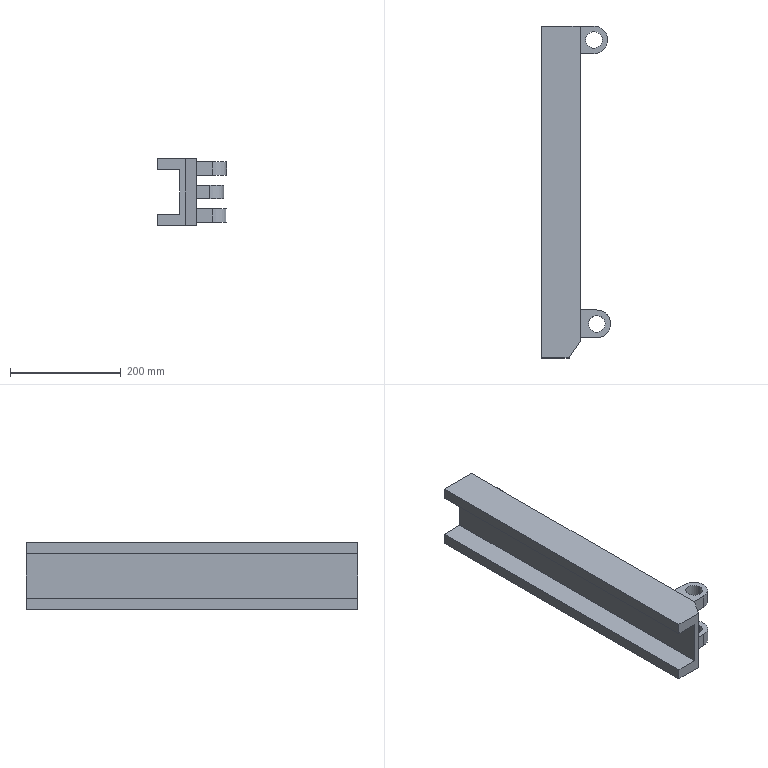Part | SolidWorks | features ICE 4, MirrorPattern 2, Extrusion 1 | 1 solid | 33 faces | box 125 x 600 x 120 mm | volume 3208933 mm3 | plane 22 | cylinder 11 | commonest cylinder face diameters 30 x6 50 x5
STEP:
#1=CARTESIAN_POINT('',(60.,575.,-12.));
#2=VERTEX_POINT('',#1);
#3=CARTESIAN_POINT('',(90.,575.,-12.));
#4=VERTEX_POINT('',#3);
#5=CARTESIAN_POINT('',(75.,575.,-12.));
#6=DIRECTION('',(0.,0.,1.));
#7=DIRECTION('',(1.,0.,0.));
#8=AXIS2_PLACEMENT_3D('',#5,#6,#7);
#9=CIRCLE('',#8,15.);
#10=EDGE_CURVE('',#2,#4,#9,.T.);
#11=ORIENTED_EDGE('',*,*,#10,.F.);
#12=CARTESIAN_POINT('',(60.,575.,12.));
#13=VERTEX_POINT('',#12);
#14=CARTESIAN_POINT('',(60.,575.,-12.));
#15=DIRECTION('',(0.,0.,1.));
#16=VECTOR('',#15,1000.);
#17=LINE('',#14,#16);
#18=EDGE_CURVE('',#2,#13,#17,.T.);
#19=ORIENTED_EDGE('',*,*,#18,.T.);
#20=CARTESIAN_POINT('',(90.,575.,12.));
#21=VERTEX_POINT('',#20);
#22=CARTESIAN_POINT('',(75.,575.,12.));
#23=DIRECTION('',(0.,0.,1.));
#24=DIRECTION('',(1.,0.,0.));
#25=AXIS2_PLACEMENT_3D('',#22,#23,#24);
#26=CIRCLE('',#25,15.);
#27=EDGE_CURVE('',#13,#21,#26,.T.);
#28=ORIENTED_EDGE('',*,*,#27,.T.);
#29=CARTESIAN_POINT('',(90.,575.,-12.));
#30=DIRECTION('',(0.,0.,1.));
#31=VECTOR('',#30,1000.);
#32=LINE('',#29,#31);
#33=EDGE_CURVE('',#4,#21,#32,.T.);
#34=ORIENTED_EDGE('',*,*,#33,.F.);
#35=EDGE_LOOP('',(#11,#19,#28,#34));
#36=FACE_OUTER_BOUND('',#35,.T.);
#37=CARTESIAN_POINT('',(75.,575.,-12.));
#38=DIRECTION('',(0.,0.,1.));
#39=DIRECTION('',(1.,0.,0.));
#40=AXIS2_PLACEMENT_3D('',#37,#38,#39);
#41=CYLINDRICAL_SURFACE('',#40,15.);
#42=ADVANCED_FACE('',(#36),#41,.F.);
#43=CARTESIAN_POINT('',(75.,550.,-12.));
#44=VERTEX_POINT('',#43);
#45=CARTESIAN_POINT('',(100.,575.,-12.));
#46=VERTEX_POINT('',#45);
#47=CARTESIAN_POINT('',(75.,575.,-12.));
#48=DIRECTION('',(0.,0.,1.));
#49=DIRECTION('',(1.,0.,0.));
#50=AXIS2_PLACEMENT_3D('',#47,#48,#49);
#51=CIRCLE('',#50,25.);
#52=EDGE_CURVE('',#44,#46,#51,.T.);
#53=ORIENTED_EDGE('',*,*,#52,.T.);
#54=CARTESIAN_POINT('',(100.,575.,12.));
#55=VERTEX_POINT('',#54);
#56=CARTESIAN_POINT('',(100.,575.,-12.));
#57=DIRECTION('',(0.,0.,1.));
#58=VECTOR('',#57,1000.);
#59=LINE('',#56,#58);
#60=EDGE_CURVE('',#46,#55,#59,.T.);
#61=ORIENTED_EDGE('',*,*,#60,.T.);
#62=CARTESIAN_POINT('',(75.,550.,12.));
#63=VERTEX_POINT('',#62);
#64=CARTESIAN_POINT('',(75.,575.,12.));
#65=DIRECTION('',(0.,0.,1.));
#66=DIRECTION('',(1.,0.,0.));
#67=AXIS2_PLACEMENT_3D('',#64,#65,#66);
#68=CIRCLE('',#67,25.);
#69=EDGE_CURVE('',#63,#55,#68,.T.);
#70=ORIENTED_EDGE('',*,*,#69,.F.);
#71=CARTESIAN_POINT('',(75.,550.,-12.));
#72=DIRECTION('',(0.,0.,1.));
#73=VECTOR('',#72,1000.);
#74=LINE('',#71,#73);
#75=EDGE_CURVE('',#44,#63,#74,.T.);
#76=ORIENTED_EDGE('',*,*,#75,.F.);
#77=EDGE_LOOP('',(#53,#61,#70,#76));
#78=FACE_OUTER_BOUND('',#77,.T.);
#79=CARTESIAN_POINT('',(75.,575.,-12.));
#80=DIRECTION('',(0.,0.,1.));
#81=DIRECTION('',(1.,0.,0.));
#82=AXIS2_PLACEMENT_3D('',#79,#80,#81);
#83=CYLINDRICAL_SURFACE('',#82,25.);
#84=ADVANCED_FACE('',(#78),#83,.T.);
#85=CARTESIAN_POINT('',(95.,61.654,-30.));
#86=VERTEX_POINT('',#85);
#87=CARTESIAN_POINT('',(65.,61.654,-30.));
#88=VERTEX_POINT('',#87);
#89=CARTESIAN_POINT('',(80.,61.654,-30.));
#90=DIRECTION('',(0.,0.,-1.));
#91=DIRECTION('',(-1.,0.,0.));
#92=AXIS2_PLACEMENT_3D('',#89,#90,#91);
#93=CIRCLE('',#92,15.);
#94=EDGE_CURVE('',#86,#88,#93,.T.);
#95=ORIENTED_EDGE('',*,*,#94,.F.);
#96=CARTESIAN_POINT('',(95.,61.654,-55.));
#97=VERTEX_POINT('',#96);
#98=CARTESIAN_POINT('',(95.,61.654,-30.));
#99=DIRECTION('',(0.,0.,-1.));
#100=VECTOR('',#99,1000.);
#101=LINE('',#98,#100);
#102=EDGE_CURVE('',#86,#97,#101,.T.);
#103=ORIENTED_EDGE('',*,*,#102,.T.);
#104=CARTESIAN_POINT('',(65.,61.654,-55.));
#105=VERTEX_POINT('',#104);
#106=CARTESIAN_POINT('',(80.,61.654,-55.));
#107=DIRECTION('',(0.,0.,1.));
#108=DIRECTION('',(-1.,0.,0.));
#109=AXIS2_PLACEMENT_3D('',#106,#107,#108);
#110=CIRCLE('',#109,15.);
#111=EDGE_CURVE('',#105,#97,#110,.T.);
#112=ORIENTED_EDGE('',*,*,#111,.F.);
#113=CARTESIAN_POINT('',(65.,61.654,-30.));
#114=DIRECTION('',(0.,0.,-1.));
#115=VECTOR('',#114,1000.);
#116=LINE('',#113,#115);
#117=EDGE_CURVE('',#88,#105,#116,.T.);
#118=ORIENTED_EDGE('',*,*,#117,.F.);
#119=EDGE_LOOP('',(#95,#103,#112,#118));
#120=FACE_OUTER_BOUND('',#119,.T.);
#121=CARTESIAN_POINT('',(80.,61.654,-30.));
#122=DIRECTION('',(0.,0.,-1.));
#123=DIRECTION('',(-1.,0.,0.));
#124=AXIS2_PLACEMENT_3D('',#121,#122,#123);
#125=CYLINDRICAL_SURFACE('',#124,15.);
#126=ADVANCED_FACE('',(#120),#125,.F.);
#127=CARTESIAN_POINT('',(95.,61.654,30.));
#128=VERTEX_POINT('',#127);
#129=CARTESIAN_POINT('',(65.,61.654,30.));
#130=VERTEX_POINT('',#129);
#131=CARTESIAN_POINT('',(80.,61.654,30.));
#132=DIRECTION('',(0.,0.,-1.));
#133=DIRECTION('',(-1.,0.,0.));
#134=AXIS2_PLACEMENT_3D('',#131,#132,#133);
#135=CIRCLE('',#134,15.);
#136=EDGE_CURVE('',#128,#130,#135,.T.);
#137=ORIENTED_EDGE('',*,*,#136,.T.);
#138=CARTESIAN_POINT('',(65.,61.654,55.));
#139=VERTEX_POINT('',#138);
#140=CARTESIAN_POINT('',(65.,61.654,30.));
#141=DIRECTION('',(0.,0.,1.));
#142=VECTOR('',#141,1000.);
#143=LINE('',#140,#142);
#144=EDGE_CURVE('',#130,#139,#143,.T.);
#145=ORIENTED_EDGE('',*,*,#144,.T.);
#146=CARTESIAN_POINT('',(95.,61.654,55.));
#147=VERTEX_POINT('',#146);
#148=CARTESIAN_POINT('',(80.,61.654,55.));
#149=DIRECTION('',(0.,0.,1.));
#150=DIRECTION('',(1.,0.,0.));
#151=AXIS2_PLACEMENT_3D('',#148,#149,#150);
#152=CIRCLE('',#151,15.);
#153=EDGE_CURVE('',#139,#147,#152,.T.);
#154=ORIENTED_EDGE('',*,*,#153,.T.);
#155=CARTESIAN_POINT('',(95.,61.654,30.));
#156=DIRECTION('',(0.,0.,1.));
#157=VECTOR('',#156,1000.);
#158=LINE('',#155,#157);
#159=EDGE_CURVE('',#128,#147,#158,.T.);
#160=ORIENTED_EDGE('',*,*,#159,.F.);
#161=EDGE_LOOP('',(#137,#145,#154,#160));
#162=FACE_OUTER_BOUND('',#161,.T.);
#163=CARTESIAN_POINT('',(80.,61.654,30.));
#164=DIRECTION('',(0.,0.,1.));
#165=DIRECTION('',(1.,0.,0.));
#166=AXIS2_PLACEMENT_3D('',#163,#164,#165);
#167=CYLINDRICAL_SURFACE('',#166,15.);
#168=ADVANCED_FACE('',(#162),#167,.F.);
#169=CARTESIAN_POINT('',(105.,61.654,30.));
#170=VERTEX_POINT('',#169);
#171=CARTESIAN_POINT('',(80.,36.654,30.));
#172=VERTEX_POINT('',#171);
#173=CARTESIAN_POINT('',(80.,61.654,30.));
#174=DIRECTION('',(0.,0.,-1.));
#175=DIRECTION('',(-1.,0.,0.));
#176=AXIS2_PLACEMENT_3D('',#173,#174,#175);
#177=CIRCLE('',#176,25.);
#178=EDGE_CURVE('',#170,#172,#177,.T.);
#179=ORIENTED_EDGE('',*,*,#178,.F.);
#180=CARTESIAN_POINT('',(105.,61.654,55.));
#181=VERTEX_POINT('',#180);
#182=CARTESIAN_POINT('',(105.,61.654,30.));
#183=DIRECTION('',(0.,0.,1.));
#184=VECTOR('',#183,1000.);
#185=LINE('',#182,#184);
#186=EDGE_CURVE('',#170,#181,#185,.T.);
#187=ORIENTED_EDGE('',*,*,#186,.T.);
#188=CARTESIAN_POINT('',(80.,36.654,55.));
#189=VERTEX_POINT('',#188);
#190=CARTESIAN_POINT('',(80.,61.654,55.));
#191=DIRECTION('',(0.,0.,1.));
#192=DIRECTION('',(1.,0.,0.));
#193=AXIS2_PLACEMENT_3D('',#190,#191,#192);
#194=CIRCLE('',#193,25.);
#195=EDGE_CURVE('',#189,#181,#194,.T.);
#196=ORIENTED_EDGE('',*,*,#195,.F.);
#197=CARTESIAN_POINT('',(80.,36.654,30.));
#198=DIRECTION('',(0.,0.,1.));
#199=VECTOR('',#198,1000.);
#200=LINE('',#197,#199);
#201=EDGE_CURVE('',#172,#189,#200,.T.);
#202=ORIENTED_EDGE('',*,*,#201,.F.);
#203=EDGE_LOOP('',(#179,#187,#196,#202));
#204=FACE_OUTER_BOUND('',#203,.T.);
#205=CARTESIAN_POINT('',(80.,61.654,30.));
#206=DIRECTION('',(0.,0.,1.));
#207=DIRECTION('',(1.,0.,0.));
#208=AXIS2_PLACEMENT_3D('',#205,#206,#207);
#209=CYLINDRICAL_SURFACE('',#208,25.);
#210=ADVANCED_FACE('',(#204),#209,.T.);
#211=CARTESIAN_POINT('',(-20.,0.,60.));
#212=VERTEX_POINT('',#211);
#213=CARTESIAN_POINT('',(30.,0.,60.));
#214=VERTEX_POINT('',#213);
#215=CARTESIAN_POINT('',(-20.,0.,60.));
#216=DIRECTION('',(1.,0.,0.));
#217=VECTOR('',#216,1000.);
#218=LINE('',#215,#217);
#219=EDGE_CURVE('',#212,#214,#218,.T.);
#220=ORIENTED_EDGE('',*,*,#219,.T.);
#221=CARTESIAN_POINT('',(50.,30.341,60.));
#222=VERTEX_POINT('',#221);
#223=CARTESIAN_POINT('',(50.,30.341,60.));
#224=DIRECTION('',(0.5504,0.8349,0.));
#225=VECTOR('',#224,1000.);
#226=LINE('',#223,#225);
#227=EDGE_CURVE('',#214,#222,#226,.T.);
#228=ORIENTED_EDGE('',*,*,#227,.T.);
#229=CARTESIAN_POINT('',(50.,600.,60.));
#230=VERTEX_POINT('',#229);
#231=CARTESIAN_POINT('',(50.,600.,60.));
#232=DIRECTION('',(0.,-1.,0.));
#233=VECTOR('',#232,1000.);
#234=LINE('',#231,#233);
#235=EDGE_CURVE('',#230,#222,#234,.T.);
#236=ORIENTED_EDGE('',*,*,#235,.F.);
#237=CARTESIAN_POINT('',(-20.,600.,60.));
#238=VERTEX_POINT('',#237);
#239=CARTESIAN_POINT('',(-20.,600.,60.));
#240=DIRECTION('',(1.,0.,0.));
#241=VECTOR('',#240,1000.);
#242=LINE('',#239,#241);
#243=EDGE_CURVE('',#238,#230,#242,.T.);
#244=ORIENTED_EDGE('',*,*,#243,.F.);
#245=CARTESIAN_POINT('',(-20.,600.,60.));
#246=DIRECTION('',(0.,-1.,0.));
#247=VECTOR('',#246,1000.);
#248=LINE('',#245,#247);
#249=EDGE_CURVE('',#238,#212,#248,.T.);
#250=ORIENTED_EDGE('',*,*,#249,.T.);
#251=EDGE_LOOP('',(#220,#228,#236,#244,#250));
#252=FACE_OUTER_BOUND('',#251,.T.);
#253=CARTESIAN_POINT('',(-20.,600.,60.));
#254=DIRECTION('',(0.,0.,-1.));
#255=DIRECTION('',(-1.,0.,0.));
#256=AXIS2_PLACEMENT_3D('',#253,#254,#255);
#257=PLANE('',#256);
#258=ADVANCED_FACE('',(#252),#257,.F.);
#259=CARTESIAN_POINT('',(50.,36.654,55.));
#260=VERTEX_POINT('',#259);
#261=CARTESIAN_POINT('',(50.,36.654,55.));
#262=DIRECTION('',(-1.,0.,0.));
#263=VECTOR('',#262,1000.);
#264=LINE('',#261,#263);
#265=EDGE_CURVE('',#189,#260,#264,.T.);
#266=ORIENTED_EDGE('',*,*,#265,.T.);
#267=CARTESIAN_POINT('',(50.,36.654,30.));
#268=VERTEX_POINT('',#267);
#269=CARTESIAN_POINT('',(50.,36.654,-60.));
#270=DIRECTION('',(0.,0.,-1.));
#271=VECTOR('',#270,1000.);
#272=LINE('',#269,#271);
#273=EDGE_CURVE('',#260,#268,#272,.T.);
#274=ORIENTED_EDGE('',*,*,#273,.T.);
#275=CARTESIAN_POINT('',(34.984,36.654,30.));
#276=DIRECTION('',(-1.,0.,0.));
#277=VECTOR('',#276,1000.);
#278=LINE('',#275,#277);
#279=EDGE_CURVE('',#172,#268,#278,.T.);
#280=ORIENTED_EDGE('',*,*,#279,.F.);
#281=ORIENTED_EDGE('',*,*,#201,.T.);
#282=EDGE_LOOP('',(#266,#274,#280,#281));
#283=FACE_OUTER_BOUND('',#282,.T.);
#284=CARTESIAN_POINT('',(34.984,36.654,30.));
#285=DIRECTION('',(0.,1.,0.));
#286=DIRECTION('',(0.,0.,1.));
#287=AXIS2_PLACEMENT_3D('',#284,#285,#286);
#288=PLANE('',#287);
#289=ADVANCED_FACE('',(#283),#288,.F.);
#290=CARTESIAN_POINT('',(80.,86.654,55.));
#291=VERTEX_POINT('',#290);
#292=CARTESIAN_POINT('',(50.,86.654,55.));
#293=VERTEX_POINT('',#292);
#294=CARTESIAN_POINT('',(34.984,86.654,55.));
#295=DIRECTION('',(-1.,0.,0.));
#296=VECTOR('',#295,1000.);
#297=LINE('',#294,#296);
#298=EDGE_CURVE('',#291,#293,#297,.T.);
#299=ORIENTED_EDGE('',*,*,#298,.F.);
#300=CARTESIAN_POINT('',(80.,86.654,30.));
#301=VERTEX_POINT('',#300);
#302=CARTESIAN_POINT('',(80.,86.654,30.));
#303=DIRECTION('',(0.,0.,1.));
#304=VECTOR('',#303,1000.);
#305=LINE('',#302,#304);
#306=EDGE_CURVE('',#301,#291,#305,.T.);
#307=ORIENTED_EDGE('',*,*,#306,.F.);
#308=CARTESIAN_POINT('',(50.,86.654,30.));
#309=VERTEX_POINT('',#308);
#310=CARTESIAN_POINT('',(34.984,86.654,30.));
#311=DIRECTION('',(1.,0.,0.));
#312=VECTOR('',#311,1000.);
#313=LINE('',#310,#312);
#314=EDGE_CURVE('',#309,#301,#313,.T.);
#315=ORIENTED_EDGE('',*,*,#314,.F.);
#316=CARTESIAN_POINT('',(50.,86.654,-60.));
#317=DIRECTION('',(0.,0.,1.));
#318=VECTOR('',#317,1000.);
#319=LINE('',#316,#318);
#320=EDGE_CURVE('',#309,#293,#319,.T.);
#321=ORIENTED_EDGE('',*,*,#320,.T.);
#322=EDGE_LOOP('',(#299,#307,#315,#321));
#323=FACE_OUTER_BOUND('',#322,.T.);
#324=CARTESIAN_POINT('',(34.984,86.654,30.));
#325=DIRECTION('',(0.,-1.,0.));
#326=DIRECTION('',(0.,0.,-1.));
#327=AXIS2_PLACEMENT_3D('',#324,#325,#326);
#328=PLANE('',#327);
#329=ADVANCED_FACE('',(#323),#328,.F.);
#330=ORIENTED_EDGE('',*,*,#186,.F.);
#331=CARTESIAN_POINT('',(80.,61.654,30.));
#332=DIRECTION('',(0.,0.,-1.));
#333=DIRECTION('',(-1.,0.,0.));
#334=AXIS2_PLACEMENT_3D('',#331,#332,#333);
#335=CIRCLE('',#334,25.);
#336=EDGE_CURVE('',#301,#170,#335,.T.);
#337=ORIENTED_EDGE('',*,*,#336,.F.);
#338=ORIENTED_EDGE('',*,*,#306,.T.);
#339=CARTESIAN_POINT('',(80.,61.654,55.));
#340=DIRECTION('',(0.,0.,1.));
#341=DIRECTION('',(1.,0.,0.));
#342=AXIS2_PLACEMENT_3D('',#339,#340,#341);
#343=CIRCLE('',#342,25.);
#344=EDGE_CURVE('',#181,#291,#343,.T.);
#345=ORIENTED_EDGE('',*,*,#344,.F.);
#346=EDGE_LOOP('',(#330,#337,#338,#345));
#347=FACE_OUTER_BOUND('',#346,.T.);
#348=CARTESIAN_POINT('',(80.,61.654,30.));
#349=DIRECTION('',(0.,0.,1.));
#350=DIRECTION('',(1.,0.,0.));
#351=AXIS2_PLACEMENT_3D('',#348,#349,#350);
#352=CYLINDRICAL_SURFACE('',#351,25.);
#353=ADVANCED_FACE('',(#347),#352,.T.);
#354=ORIENTED_EDGE('',*,*,#144,.F.);
#355=CARTESIAN_POINT('',(80.,61.654,30.));
#356=DIRECTION('',(0.,0.,-1.));
#357=DIRECTION('',(-1.,0.,0.));
#358=AXIS2_PLACEMENT_3D('',#355,#356,#357);
#359=CIRCLE('',#358,15.);
#360=EDGE_CURVE('',#130,#128,#359,.T.);
#361=ORIENTED_EDGE('',*,*,#360,.T.);
#362=ORIENTED_EDGE('',*,*,#159,.T.);
#363=CARTESIAN_POINT('',(80.,61.654,55.));
#364=DIRECTION('',(0.,0.,1.));
#365=DIRECTION('',(1.,0.,0.));
#366=AXIS2_PLACEMENT_3D('',#363,#364,#365);
#367=CIRCLE('',#366,15.);
#368=EDGE_CURVE('',#147,#139,#367,.T.);
#369=ORIENTED_EDGE('',*,*,#368,.T.);
#370=EDGE_LOOP('',(#354,#361,#362,#369));
#371=FACE_OUTER_BOUND('',#370,.T.);
#372=CARTESIAN_POINT('',(80.,61.654,30.));
#373=DIRECTION('',(0.,0.,1.));
#374=DIRECTION('',(1.,0.,0.));
#375=AXIS2_PLACEMENT_3D('',#372,#373,#374);
#376=CYLINDRICAL_SURFACE('',#375,15.);
#377=ADVANCED_FACE('',(#371),#376,.F.);
#378=CARTESIAN_POINT('',(80.,86.654,-30.));
#379=VERTEX_POINT('',#378);
#380=CARTESIAN_POINT('',(80.,86.654,-55.));
#381=VERTEX_POINT('',#380);
#382=CARTESIAN_POINT('',(80.,86.654,-30.));
#383=DIRECTION('',(0.,0.,-1.));
#384=VECTOR('',#383,1000.);
#385=LINE('',#382,#384);
#386=EDGE_CURVE('',#379,#381,#385,.T.);
#387=ORIENTED_EDGE('',*,*,#386,.T.);
#388=CARTESIAN_POINT('',(50.,86.654,-55.));
#389=VERTEX_POINT('',#388);
#390=CARTESIAN_POINT('',(34.984,86.654,-55.));
#391=DIRECTION('',(-1.,0.,0.));
#392=VECTOR('',#391,1000.);
#393=LINE('',#390,#392);
#394=EDGE_CURVE('',#381,#389,#393,.T.);
#395=ORIENTED_EDGE('',*,*,#394,.T.);
#396=CARTESIAN_POINT('',(50.,86.654,-30.));
#397=VERTEX_POINT('',#396);
#398=CARTESIAN_POINT('',(50.,86.654,-60.));
#399=DIRECTION('',(0.,0.,-1.));
#400=VECTOR('',#399,1000.);
#401=LINE('',#398,#400);
#402=EDGE_CURVE('',#397,#389,#401,.T.);
#403=ORIENTED_EDGE('',*,*,#402,.F.);
#404=CARTESIAN_POINT('',(34.984,86.654,-30.));
#405=DIRECTION('',(1.,0.,0.));
#406=VECTOR('',#405,1000.);
#407=LINE('',#404,#406);
#408=EDGE_CURVE('',#397,#379,#407,.T.);
#409=ORIENTED_EDGE('',*,*,#408,.T.);
#410=EDGE_LOOP('',(#387,#395,#403,#409));
#411=FACE_OUTER_BOUND('',#410,.T.);
#412=CARTESIAN_POINT('',(34.984,86.654,-30.));
#413=DIRECTION('',(0.,1.,0.));
#414=DIRECTION('',(0.,0.,1.));
#415=AXIS2_PLACEMENT_3D('',#412,#413,#414);
#416=PLANE('',#415);
#417=ADVANCED_FACE('',(#411),#416,.T.);
#418=CARTESIAN_POINT('',(50.,36.654,-55.));
#419=VERTEX_POINT('',#418);
#420=CARTESIAN_POINT('',(50.,36.654,-30.));
#421=VERTEX_POINT('',#420);
#422=CARTESIAN_POINT('',(50.,36.654,-60.));
#423=DIRECTION('',(0.,0.,1.));
#424=VECTOR('',#423,1000.);
#425=LINE('',#422,#424);
#426=EDGE_CURVE('',#419,#421,#425,.T.);
#427=ORIENTED_EDGE('',*,*,#426,.F.);
#428=CARTESIAN_POINT('',(80.,36.654,-55.));
#429=VERTEX_POINT('',#428);
#430=CARTESIAN_POINT('',(50.,36.654,-55.));
#431=DIRECTION('',(-1.,0.,0.));
#432=VECTOR('',#431,1000.);
#433=LINE('',#430,#432);
#434=EDGE_CURVE('',#429,#419,#433,.T.);
#435=ORIENTED_EDGE('',*,*,#434,.F.);
#436=CARTESIAN_POINT('',(80.,36.654,-30.));
#437=VERTEX_POINT('',#436);
#438=CARTESIAN_POINT('',(80.,36.654,-30.));
#439=DIRECTION('',(0.,0.,-1.));
#440=VECTOR('',#439,1000.);
#441=LINE('',#438,#440);
#442=EDGE_CURVE('',#437,#429,#441,.T.);
#443=ORIENTED_EDGE('',*,*,#442,.F.);
#444=CARTESIAN_POINT('',(34.984,36.654,-30.));
#445=DIRECTION('',(-1.,0.,0.));
#446=VECTOR('',#445,1000.);
#447=LINE('',#444,#446);
#448=EDGE_CURVE('',#437,#421,#447,.T.);
#449=ORIENTED_EDGE('',*,*,#448,.T.);
#450=EDGE_LOOP('',(#427,#435,#443,#449));
#451=FACE_OUTER_BOUND('',#450,.T.);
#452=CARTESIAN_POINT('',(34.984,36.654,-30.));
#453=DIRECTION('',(0.,-1.,0.));
#454=DIRECTION('',(0.,0.,-1.));
#455=AXIS2_PLACEMENT_3D('',#452,#453,#454);
#456=PLANE('',#455);
#457=ADVANCED_FACE('',(#451),#456,.T.);
#458=ORIENTED_EDGE('',*,*,#442,.T.);
#459=CARTESIAN_POINT('',(80.,61.654,-55.));
#460=DIRECTION('',(0.,0.,1.));
#461=DIRECTION('',(-1.,0.,0.));
#462=AXIS2_PLACEMENT_3D('',#459,#460,#461);
#463=CIRCLE('',#462,25.);
#464=EDGE_CURVE('',#429,#381,#463,.T.);
#465=ORIENTED_EDGE('',*,*,#464,.T.);
#466=ORIENTED_EDGE('',*,*,#386,.F.);
#467=CARTESIAN_POINT('',(80.,61.654,-30.));
#468=DIRECTION('',(0.,0.,-1.));
#469=DIRECTION('',(-1.,0.,0.));
#470=AXIS2_PLACEMENT_3D('',#467,#468,#469);
#471=CIRCLE('',#470,25.);
#472=EDGE_CURVE('',#379,#437,#471,.T.);
#473=ORIENTED_EDGE('',*,*,#472,.T.);
#474=EDGE_LOOP('',(#458,#465,#466,#473));
#475=FACE_OUTER_BOUND('',#474,.T.);
#476=CARTESIAN_POINT('',(80.,61.654,-30.));
#477=DIRECTION('',(0.,0.,-1.));
#478=DIRECTION('',(-1.,0.,0.));
#479=AXIS2_PLACEMENT_3D('',#476,#477,#478);
#480=CYLINDRICAL_SURFACE('',#479,25.);
#481=ADVANCED_FACE('',(#475),#480,.T.);
#482=ORIENTED_EDGE('',*,*,#102,.F.);
#483=CARTESIAN_POINT('',(80.,61.654,-30.));
#484=DIRECTION('',(0.,0.,-1.));
#485=DIRECTION('',(-1.,0.,0.));
#486=AXIS2_PLACEMENT_3D('',#483,#484,#485);
#487=CIRCLE('',#486,15.);
#488=EDGE_CURVE('',#88,#86,#487,.T.);
#489=ORIENTED_EDGE('',*,*,#488,.F.);
#490=ORIENTED_EDGE('',*,*,#117,.T.);
#491=CARTESIAN_POINT('',(80.,61.654,-55.));
#492=DIRECTION('',(0.,0.,1.));
#493=DIRECTION('',(-1.,0.,0.));
#494=AXIS2_PLACEMENT_3D('',#491,#492,#493);
#495=CIRCLE('',#494,15.);
#496=EDGE_CURVE('',#97,#105,#495,.T.);
#497=ORIENTED_EDGE('',*,*,#496,.F.);
#498=EDGE_LOOP('',(#482,#489,#490,#497));
#499=FACE_OUTER_BOUND('',#498,.T.);
#500=CARTESIAN_POINT('',(80.,61.654,-30.));
#501=DIRECTION('',(0.,0.,-1.));
#502=DIRECTION('',(-1.,0.,0.));
#503=AXIS2_PLACEMENT_3D('',#500,#501,#502);
#504=CYLINDRICAL_SURFACE('',#503,15.);
#505=ADVANCED_FACE('',(#499),#504,.F.);
#506=ORIENTED_EDGE('',*,*,#235,.T.);
#507=CARTESIAN_POINT('',(50.,30.341,-60.));
#508=VERTEX_POINT('',#507);
#509=CARTESIAN_POINT('',(50.,30.341,60.));
#510=DIRECTION('',(0.,0.,-1.));
#511=VECTOR('',#510,1000.);
#512=LINE('',#509,#511);
#513=EDGE_CURVE('',#222,#508,#512,.T.);
#514=ORIENTED_EDGE('',*,*,#513,.T.);
#515=CARTESIAN_POINT('',(50.,600.,-60.));
#516=VERTEX_POINT('',#515);
#517=CARTESIAN_POINT('',(50.,600.,-60.));
#518=DIRECTION('',(0.,-1.,0.));
#519=VECTOR('',#518,1000.);
#520=LINE('',#517,#519);
#521=EDGE_CURVE('',#516,#508,#520,.T.);
#522=ORIENTED_EDGE('',*,*,#521,.F.);
#523=CARTESIAN_POINT('',(50.,600.,-12.));
#524=VERTEX_POINT('',#523);
#525=CARTESIAN_POINT('',(50.,600.,-60.));
#526=DIRECTION('',(0.,0.,-1.));
#527=VECTOR('',#526,1000.);
#528=LINE('',#525,#527);
#529=EDGE_CURVE('',#524,#516,#528,.T.);
#530=ORIENTED_EDGE('',*,*,#529,.F.);
#531=CARTESIAN_POINT('',(50.,550.,-12.));
#532=VERTEX_POINT('',#531);
#533=CARTESIAN_POINT('',(50.,600.,-12.));
#534=DIRECTION('',(0.,1.,0.));
#535=VECTOR('',#534,1000.);
#536=LINE('',#533,#535);
#537=EDGE_CURVE('',#532,#524,#536,.T.);
#538=ORIENTED_EDGE('',*,*,#537,.F.);
#539=CARTESIAN_POINT('',(50.,550.,12.));
#540=VERTEX_POINT('',#539);
#541=CARTESIAN_POINT('',(50.,550.,-60.));
#542=DIRECTION('',(0.,0.,1.));
#543=VECTOR('',#542,1000.);
#544=LINE('',#541,#543);
#545=EDGE_CURVE('',#532,#540,#544,.T.);
#546=ORIENTED_EDGE('',*,*,#545,.T.);
#547=CARTESIAN_POINT('',(50.,600.,12.));
#548=VERTEX_POINT('',#547);
#549=CARTESIAN_POINT('',(50.,600.,12.));
#550=DIRECTION('',(0.,1.,0.));
#551=VECTOR('',#550,1000.);
#552=LINE('',#549,#551);
#553=EDGE_CURVE('',#540,#548,#552,.T.);
#554=ORIENTED_EDGE('',*,*,#553,.T.);
#555=CARTESIAN_POINT('',(50.,600.,-60.));
#556=DIRECTION('',(0.,0.,-1.));
#557=VECTOR('',#556,1000.);
#558=LINE('',#555,#557);
#559=EDGE_CURVE('',#230,#548,#558,.T.);
#560=ORIENTED_EDGE('',*,*,#559,.F.);
#561=EDGE_LOOP('',(#506,#514,#522,#530,#538,#546,#554,#560));
#562=FACE_OUTER_BOUND('',#561,.T.);
#563=CARTESIAN_POINT('',(50.,36.654,55.));
#564=DIRECTION('',(0.,1.,0.));
#565=VECTOR('',#564,1000.);
#566=LINE('',#563,#565);
#567=EDGE_CURVE('',#260,#293,#566,.T.);
#568=ORIENTED_EDGE('',*,*,#567,.T.);
#569=ORIENTED_EDGE('',*,*,#320,.F.);
#570=CARTESIAN_POINT('',(50.,600.,30.));
#571=DIRECTION('',(0.,1.,0.));
#572=VECTOR('',#571,1000.);
#573=LINE('',#570,#572);
#574=EDGE_CURVE('',#268,#309,#573,.T.);
#575=ORIENTED_EDGE('',*,*,#574,.F.);
#576=ORIENTED_EDGE('',*,*,#273,.F.);
#577=EDGE_LOOP('',(#568,#569,#575,#576));
#578=FACE_BOUND('',#577,.T.);
#579=ORIENTED_EDGE('',*,*,#402,.T.);
#580=CARTESIAN_POINT('',(50.,36.654,-55.));
#581=DIRECTION('',(0.,1.,0.));
#582=VECTOR('',#581,1000.);
#583=LINE('',#580,#582);
#584=EDGE_CURVE('',#419,#389,#583,.T.);
#585=ORIENTED_EDGE('',*,*,#584,.F.);
#586=ORIENTED_EDGE('',*,*,#426,.T.);
#587=CARTESIAN_POINT('',(50.,600.,-30.));
#588=DIRECTION('',(0.,-1.,0.));
#589=VECTOR('',#588,1000.);
#590=LINE('',#587,#589);
#591=EDGE_CURVE('',#397,#421,#590,.T.);
#592=ORIENTED_EDGE('',*,*,#591,.F.);
#593=EDGE_LOOP('',(#579,#585,#586,#592));
#594=FACE_BOUND('',#593,.T.);
#595=CARTESIAN_POINT('',(50.,600.,-60.));
#596=DIRECTION('',(-1.,0.,0.));
#597=DIRECTION('',(0.,0.,1.));
#598=AXIS2_PLACEMENT_3D('',#595,#596,#597);
#599=PLANE('',#598);
#600=ADVANCED_FACE('',(#562,#578,#594),#599,.F.);
#601=CARTESIAN_POINT('',(20.,0.,-40.));
#602=VERTEX_POINT('',#601);
#603=CARTESIAN_POINT('',(20.,0.,40.));
#604=VERTEX_POINT('',#603);
#605=CARTESIAN_POINT('',(20.,0.,-40.));
#606=DIRECTION('',(0.,0.,1.));
#607=VECTOR('',#606,1000.);
#608=LINE('',#605,#607);
#609=EDGE_CURVE('',#602,#604,#608,.T.);
#610=ORIENTED_EDGE('',*,*,#609,.T.);
#611=CARTESIAN_POINT('',(20.,600.,40.));
#612=VERTEX_POINT('',#611);
#613=CARTESIAN_POINT('',(20.,600.,40.));
#614=DIRECTION('',(0.,-1.,0.));
#615=VECTOR('',#614,1000.);
#616=LINE('',#613,#615);
#617=EDGE_CURVE('',#612,#604,#616,.T.);
#618=ORIENTED_EDGE('',*,*,#617,.F.);
#619=CARTESIAN_POINT('',(20.,600.,-40.));
#620=VERTEX_POINT('',#619);
#621=CARTESIAN_POINT('',(20.,600.,-40.));
#622=DIRECTION('',(0.,0.,1.));
#623=VECTOR('',#622,1000.);
#624=LINE('',#621,#623);
#625=EDGE_CURVE('',#620,#612,#624,.T.);
#626=ORIENTED_EDGE('',*,*,#625,.F.);
#627=CARTESIAN_POINT('',(20.,600.,-40.));
#628=DIRECTION('',(0.,-1.,0.));
#629=VECTOR('',#628,1000.);
#630=LINE('',#627,#629);
#631=EDGE_CURVE('',#620,#602,#630,.T.);
#632=ORIENTED_EDGE('',*,*,#631,.T.);
#633=EDGE_LOOP('',(#610,#618,#626,#632));
#634=FACE_OUTER_BOUND('',#633,.T.);
#635=CARTESIAN_POINT('',(20.,600.,-40.));
#636=DIRECTION('',(1.,0.,0.));
#637=DIRECTION('',(0.,0.,-1.));
#638=AXIS2_PLACEMENT_3D('',#635,#636,#637);
#639=PLANE('',#638);
#640=ADVANCED_FACE('',(#634),#639,.F.);
#641=CARTESIAN_POINT('',(-20.,0.,40.));
#642=VERTEX_POINT('',#641);
#643=CARTESIAN_POINT('',(-20.,0.,40.));
#644=DIRECTION('',(-1.,0.,0.));
#645=VECTOR('',#644,1000.);
#646=LINE('',#643,#645);
#647=EDGE_CURVE('',#604,#642,#646,.T.);
#648=ORIENTED_EDGE('',*,*,#647,.T.);
#649=CARTESIAN_POINT('',(-20.,600.,40.));
#650=VERTEX_POINT('',#649);
#651=CARTESIAN_POINT('',(-20.,600.,40.));
#652=DIRECTION('',(0.,-1.,0.));
#653=VECTOR('',#652,1000.);
#654=LINE('',#651,#653);
#655=EDGE_CURVE('',#650,#642,#654,.T.);
#656=ORIENTED_EDGE('',*,*,#655,.F.);
#657=CARTESIAN_POINT('',(-20.,600.,40.));
#658=DIRECTION('',(-1.,0.,0.));
#659=VECTOR('',#658,1000.);
#660=LINE('',#657,#659);
#661=EDGE_CURVE('',#612,#650,#660,.T.);
#662=ORIENTED_EDGE('',*,*,#661,.F.);
#663=ORIENTED_EDGE('',*,*,#617,.T.);
#664=EDGE_LOOP('',(#648,#656,#662,#663));
#665=FACE_OUTER_BOUND('',#664,.T.);
#666=CARTESIAN_POINT('',(-20.,600.,40.));
#667=DIRECTION('',(0.,0.,1.));
#668=DIRECTION('',(1.,0.,0.));
#669=AXIS2_PLACEMENT_3D('',#666,#667,#668);
#670=PLANE('',#669);
#671=ADVANCED_FACE('',(#665),#670,.F.);
#672=CARTESIAN_POINT('',(-20.,0.,40.));
#673=DIRECTION('',(0.,0.,1.));
#674=VECTOR('',#673,1000.);
#675=LINE('',#672,#674);
#676=EDGE_CURVE('',#642,#212,#675,.T.);
#677=ORIENTED_EDGE('',*,*,#676,.T.);
#678=ORIENTED_EDGE('',*,*,#249,.F.);
#679=CARTESIAN_POINT('',(-20.,600.,40.));
#680=DIRECTION('',(0.,0.,1.));
#681=VECTOR('',#680,1000.);
#682=LINE('',#679,#681);
#683=EDGE_CURVE('',#650,#238,#682,.T.);
#684=ORIENTED_EDGE('',*,*,#683,.F.);
#685=ORIENTED_EDGE('',*,*,#655,.T.);
#686=EDGE_LOOP('',(#677,#678,#684,#685));
#687=FACE_OUTER_BOUND('',#686,.T.);
#688=CARTESIAN_POINT('',(-20.,600.,40.));
#689=DIRECTION('',(1.,0.,0.));
#690=DIRECTION('',(0.,0.,-1.));
#691=AXIS2_PLACEMENT_3D('',#688,#689,#690);
#692=PLANE('',#691);
#693=ADVANCED_FACE('',(#687),#692,.F.);
#694=ORIENTED_EDGE('',*,*,#521,.T.);
#695=CARTESIAN_POINT('',(30.,0.,-60.));
#696=VERTEX_POINT('',#695);
#697=CARTESIAN_POINT('',(50.,30.341,-60.));
#698=DIRECTION('',(0.5504,0.8349,0.));
#699=VECTOR('',#698,1000.);
#700=LINE('',#697,#699);
#701=EDGE_CURVE('',#696,#508,#700,.T.);
#702=ORIENTED_EDGE('',*,*,#701,.F.);
#703=CARTESIAN_POINT('',(-20.,0.,-60.));
#704=VERTEX_POINT('',#703);
#705=CARTESIAN_POINT('',(-20.,0.,-60.));
#706=DIRECTION('',(-1.,0.,0.));
#707=VECTOR('',#706,1000.);
#708=LINE('',#705,#707);
#709=EDGE_CURVE('',#696,#704,#708,.T.);
#710=ORIENTED_EDGE('',*,*,#709,.T.);
#711=CARTESIAN_POINT('',(-20.,600.,-60.));
#712=VERTEX_POINT('',#711);
#713=CARTESIAN_POINT('',(-20.,600.,-60.));
#714=DIRECTION('',(0.,-1.,0.));
#715=VECTOR('',#714,1000.);
#716=LINE('',#713,#715);
#717=EDGE_CURVE('',#712,#704,#716,.T.);
#718=ORIENTED_EDGE('',*,*,#717,.F.);
#719=CARTESIAN_POINT('',(-20.,600.,-60.));
#720=DIRECTION('',(-1.,0.,0.));
#721=VECTOR('',#720,1000.);
#722=LINE('',#719,#721);
#723=EDGE_CURVE('',#516,#712,#722,.T.);
#724=ORIENTED_EDGE('',*,*,#723,.F.);
#725=EDGE_LOOP('',(#694,#702,#710,#718,#724));
#726=FACE_OUTER_BOUND('',#725,.T.);
#727=CARTESIAN_POINT('',(-20.,600.,-60.));
#728=DIRECTION('',(0.,0.,1.));
#729=DIRECTION('',(1.,0.,0.));
#730=AXIS2_PLACEMENT_3D('',#727,#728,#729);
#731=PLANE('',#730);
#732=ADVANCED_FACE('',(#726),#731,.F.);
#733=CARTESIAN_POINT('',(-20.,0.,-40.));
#734=VERTEX_POINT('',#733);
#735=CARTESIAN_POINT('',(-20.,0.,-40.));
#736=DIRECTION('',(0.,0.,1.));
#737=VECTOR('',#736,1000.);
#738=LINE('',#735,#737);
#739=EDGE_CURVE('',#704,#734,#738,.T.);
#740=ORIENTED_EDGE('',*,*,#739,.T.);
#741=CARTESIAN_POINT('',(-20.,600.,-40.));
#742=VERTEX_POINT('',#741);
#743=CARTESIAN_POINT('',(-20.,600.,-40.));
#744=DIRECTION('',(0.,-1.,0.));
#745=VECTOR('',#744,1000.);
#746=LINE('',#743,#745);
#747=EDGE_CURVE('',#742,#734,#746,.T.);
#748=ORIENTED_EDGE('',*,*,#747,.F.);
#749=CARTESIAN_POINT('',(-20.,600.,-40.));
#750=DIRECTION('',(0.,0.,1.));
#751=VECTOR('',#750,1000.);
#752=LINE('',#749,#751);
#753=EDGE_CURVE('',#712,#742,#752,.T.);
#754=ORIENTED_EDGE('',*,*,#753,.F.);
#755=ORIENTED_EDGE('',*,*,#717,.T.);
#756=EDGE_LOOP('',(#740,#748,#754,#755));
#757=FACE_OUTER_BOUND('',#756,.T.);
#758=CARTESIAN_POINT('',(-20.,600.,-40.));
#759=DIRECTION('',(1.,0.,0.));
#760=DIRECTION('',(0.,0.,-1.));
#761=AXIS2_PLACEMENT_3D('',#758,#759,#760);
#762=PLANE('',#761);
#763=ADVANCED_FACE('',(#757),#762,.F.);
#764=CARTESIAN_POINT('',(-20.,0.,-40.));
#765=DIRECTION('',(1.,0.,0.));
#766=VECTOR('',#765,1000.);
#767=LINE('',#764,#766);
#768=EDGE_CURVE('',#734,#602,#767,.T.);
#769=ORIENTED_EDGE('',*,*,#768,.T.);
#770=ORIENTED_EDGE('',*,*,#631,.F.);
#771=CARTESIAN_POINT('',(-20.,600.,-40.));
#772=DIRECTION('',(1.,0.,0.));
#773=VECTOR('',#772,1000.);
#774=LINE('',#771,#773);
#775=EDGE_CURVE('',#742,#620,#774,.T.);
#776=ORIENTED_EDGE('',*,*,#775,.F.);
#777=ORIENTED_EDGE('',*,*,#747,.T.);
#778=EDGE_LOOP('',(#769,#770,#776,#777));
#779=FACE_OUTER_BOUND('',#778,.T.);
#780=CARTESIAN_POINT('',(-20.,600.,-40.));
#781=DIRECTION('',(0.,0.,-1.));
#782=DIRECTION('',(-1.,0.,0.));
#783=AXIS2_PLACEMENT_3D('',#780,#781,#782);
#784=PLANE('',#783);
#785=ADVANCED_FACE('',(#779),#784,.F.);
#786=ORIENTED_EDGE('',*,*,#559,.T.);
#787=CARTESIAN_POINT('',(75.,600.,12.));
#788=VERTEX_POINT('',#787);
#789=CARTESIAN_POINT('',(42.374,600.,12.));
#790=DIRECTION('',(-1.,0.,0.));
#791=VECTOR('',#790,1000.);
#792=LINE('',#789,#791);
#793=EDGE_CURVE('',#788,#548,#792,.T.);
#794=ORIENTED_EDGE('',*,*,#793,.F.);
#795=CARTESIAN_POINT('',(75.,600.,-12.));
#796=VERTEX_POINT('',#795);
#797=CARTESIAN_POINT('',(75.,600.,-12.));
#798=DIRECTION('',(0.,0.,1.));
#799=VECTOR('',#798,1000.);
#800=LINE('',#797,#799);
#801=EDGE_CURVE('',#796,#788,#800,.T.);
#802=ORIENTED_EDGE('',*,*,#801,.F.);
#803=CARTESIAN_POINT('',(42.374,600.,-12.));
#804=DIRECTION('',(-1.,0.,0.));
#805=VECTOR('',#804,1000.);
#806=LINE('',#803,#805);
#807=EDGE_CURVE('',#796,#524,#806,.T.);
#808=ORIENTED_EDGE('',*,*,#807,.T.);
#809=ORIENTED_EDGE('',*,*,#529,.T.);
#810=ORIENTED_EDGE('',*,*,#723,.T.);
#811=ORIENTED_EDGE('',*,*,#753,.T.);
#812=ORIENTED_EDGE('',*,*,#775,.T.);
#813=ORIENTED_EDGE('',*,*,#625,.T.);
#814=ORIENTED_EDGE('',*,*,#661,.T.);
#815=ORIENTED_EDGE('',*,*,#683,.T.);
#816=ORIENTED_EDGE('',*,*,#243,.T.);
#817=EDGE_LOOP('',(#786,#794,#802,#808,#809,#810,#811,#812,#813,#814,#815,#816));
#818=FACE_OUTER_BOUND('',#817,.T.);
#819=CARTESIAN_POINT('',(0.,600.,0.));
#820=DIRECTION('',(0.,1.,0.));
#821=DIRECTION('',(0.,0.,1.));
#822=AXIS2_PLACEMENT_3D('',#819,#820,#821);
#823=PLANE('',#822);
#824=ADVANCED_FACE('',(#818),#823,.T.);
#825=ORIENTED_EDGE('',*,*,#709,.F.);
#826=CARTESIAN_POINT('',(30.,0.,60.));
#827=DIRECTION('',(0.,0.,-1.));
#828=VECTOR('',#827,1000.);
#829=LINE('',#826,#828);
#830=EDGE_CURVE('',#214,#696,#829,.T.);
#831=ORIENTED_EDGE('',*,*,#830,.F.);
#832=ORIENTED_EDGE('',*,*,#219,.F.);
#833=ORIENTED_EDGE('',*,*,#676,.F.);
#834=ORIENTED_EDGE('',*,*,#647,.F.);
#835=ORIENTED_EDGE('',*,*,#609,.F.);
#836=ORIENTED_EDGE('',*,*,#768,.F.);
#837=ORIENTED_EDGE('',*,*,#739,.F.);
#838=EDGE_LOOP('',(#825,#831,#832,#833,#834,#835,#836,#837));
#839=FACE_OUTER_BOUND('',#838,.T.);
#840=CARTESIAN_POINT('',(0.,0.,0.));
#841=DIRECTION('',(0.,1.,0.));
#842=DIRECTION('',(0.,0.,1.));
#843=AXIS2_PLACEMENT_3D('',#840,#841,#842);
#844=PLANE('',#843);
#845=ADVANCED_FACE('',(#839),#844,.F.);
#846=ORIENTED_EDGE('',*,*,#488,.T.);
#847=ORIENTED_EDGE('',*,*,#94,.T.);
#848=EDGE_LOOP('',(#846,#847));
#849=FACE_BOUND('',#848,.T.);
#850=ORIENTED_EDGE('',*,*,#408,.F.);
#851=ORIENTED_EDGE('',*,*,#591,.T.);
#852=ORIENTED_EDGE('',*,*,#448,.F.);
#853=ORIENTED_EDGE('',*,*,#472,.F.);
#854=EDGE_LOOP('',(#850,#851,#852,#853));
#855=FACE_OUTER_BOUND('',#854,.T.);
#856=CARTESIAN_POINT('',(80.,61.654,-30.));
#857=DIRECTION('',(0.,0.,-1.));
#858=DIRECTION('',(-1.,0.,0.));
#859=AXIS2_PLACEMENT_3D('',#856,#857,#858);
#860=PLANE('',#859);
#861=ADVANCED_FACE('',(#849,#855),#860,.F.);
#862=ORIENTED_EDGE('',*,*,#136,.F.);
#863=ORIENTED_EDGE('',*,*,#360,.F.);
#864=EDGE_LOOP('',(#862,#863));
#865=FACE_BOUND('',#864,.T.);
#866=ORIENTED_EDGE('',*,*,#279,.T.);
#867=ORIENTED_EDGE('',*,*,#574,.T.);
#868=ORIENTED_EDGE('',*,*,#314,.T.);
#869=ORIENTED_EDGE('',*,*,#336,.T.);
#870=ORIENTED_EDGE('',*,*,#178,.T.);
#871=EDGE_LOOP('',(#866,#867,#868,#869,#870));
#872=FACE_OUTER_BOUND('',#871,.T.);
#873=CARTESIAN_POINT('',(80.,61.654,30.));
#874=DIRECTION('',(0.,0.,1.));
#875=DIRECTION('',(-1.,0.,0.));
#876=AXIS2_PLACEMENT_3D('',#873,#874,#875);
#877=PLANE('',#876);
#878=ADVANCED_FACE('',(#865,#872),#877,.F.);
#879=ORIENTED_EDGE('',*,*,#545,.F.);
#880=CARTESIAN_POINT('',(42.374,550.,-12.));
#881=DIRECTION('',(1.,0.,0.));
#882=VECTOR('',#881,1000.);
#883=LINE('',#880,#882);
#884=EDGE_CURVE('',#532,#44,#883,.T.);
#885=ORIENTED_EDGE('',*,*,#884,.T.);
#886=ORIENTED_EDGE('',*,*,#75,.T.);
#887=CARTESIAN_POINT('',(42.374,550.,12.));
#888=DIRECTION('',(1.,0.,0.));
#889=VECTOR('',#888,1000.);
#890=LINE('',#887,#889);
#891=EDGE_CURVE('',#540,#63,#890,.T.);
#892=ORIENTED_EDGE('',*,*,#891,.F.);
#893=EDGE_LOOP('',(#879,#885,#886,#892));
#894=FACE_OUTER_BOUND('',#893,.T.);
#895=CARTESIAN_POINT('',(42.374,550.,-12.));
#896=DIRECTION('',(0.,-1.,0.));
#897=DIRECTION('',(0.,0.,-1.));
#898=AXIS2_PLACEMENT_3D('',#895,#896,#897);
#899=PLANE('',#898);
#900=ADVANCED_FACE('',(#894),#899,.T.);
#901=CARTESIAN_POINT('',(75.,575.,-12.));
#902=DIRECTION('',(0.,0.,1.));
#903=DIRECTION('',(1.,0.,0.));
#904=AXIS2_PLACEMENT_3D('',#901,#902,#903);
#905=CIRCLE('',#904,15.);
#906=EDGE_CURVE('',#4,#2,#905,.T.);
#907=ORIENTED_EDGE('',*,*,#906,.T.);
#908=ORIENTED_EDGE('',*,*,#10,.T.);
#909=EDGE_LOOP('',(#907,#908));
#910=FACE_BOUND('',#909,.T.);
#911=ORIENTED_EDGE('',*,*,#884,.F.);
#912=ORIENTED_EDGE('',*,*,#537,.T.);
#913=ORIENTED_EDGE('',*,*,#807,.F.);
#914=CARTESIAN_POINT('',(75.,575.,-12.));
#915=DIRECTION('',(0.,0.,1.));
#916=DIRECTION('',(1.,0.,0.));
#917=AXIS2_PLACEMENT_3D('',#914,#915,#916);
#918=CIRCLE('',#917,25.);
#919=EDGE_CURVE('',#46,#796,#918,.T.);
#920=ORIENTED_EDGE('',*,*,#919,.F.);
#921=ORIENTED_EDGE('',*,*,#52,.F.);
#922=EDGE_LOOP('',(#911,#912,#913,#920,#921));
#923=FACE_OUTER_BOUND('',#922,.T.);
#924=CARTESIAN_POINT('',(75.,575.,-12.));
#925=DIRECTION('',(0.,0.,1.));
#926=DIRECTION('',(1.,0.,0.));
#927=AXIS2_PLACEMENT_3D('',#924,#925,#926);
#928=PLANE('',#927);
#929=ADVANCED_FACE('',(#910,#923),#928,.F.);
#930=CARTESIAN_POINT('',(75.,575.,12.));
#931=DIRECTION('',(0.,0.,1.));
#932=DIRECTION('',(1.,0.,0.));
#933=AXIS2_PLACEMENT_3D('',#930,#931,#932);
#934=CIRCLE('',#933,15.);
#935=EDGE_CURVE('',#21,#13,#934,.T.);
#936=ORIENTED_EDGE('',*,*,#935,.F.);
#937=ORIENTED_EDGE('',*,*,#27,.F.);
#938=EDGE_LOOP('',(#936,#937));
#939=FACE_BOUND('',#938,.T.);
#940=ORIENTED_EDGE('',*,*,#553,.F.);
#941=ORIENTED_EDGE('',*,*,#891,.T.);
#942=ORIENTED_EDGE('',*,*,#69,.T.);
#943=CARTESIAN_POINT('',(75.,575.,12.));
#944=DIRECTION('',(0.,0.,1.));
#945=DIRECTION('',(1.,0.,0.));
#946=AXIS2_PLACEMENT_3D('',#943,#944,#945);
#947=CIRCLE('',#946,25.);
#948=EDGE_CURVE('',#55,#788,#947,.T.);
#949=ORIENTED_EDGE('',*,*,#948,.T.);
#950=ORIENTED_EDGE('',*,*,#793,.T.);
#951=EDGE_LOOP('',(#940,#941,#942,#949,#950));
#952=FACE_OUTER_BOUND('',#951,.T.);
#953=CARTESIAN_POINT('',(75.,575.,12.));
#954=DIRECTION('',(0.,0.,1.));
#955=DIRECTION('',(1.,0.,0.));
#956=AXIS2_PLACEMENT_3D('',#953,#954,#955);
#957=PLANE('',#956);
#958=ADVANCED_FACE('',(#939,#952),#957,.T.);
#959=ORIENTED_EDGE('',*,*,#60,.F.);
#960=ORIENTED_EDGE('',*,*,#919,.T.);
#961=ORIENTED_EDGE('',*,*,#801,.T.);
#962=ORIENTED_EDGE('',*,*,#948,.F.);
#963=EDGE_LOOP('',(#959,#960,#961,#962));
#964=FACE_OUTER_BOUND('',#963,.T.);
#965=CARTESIAN_POINT('',(75.,575.,-12.));
#966=DIRECTION('',(0.,0.,1.));
#967=DIRECTION('',(1.,0.,0.));
#968=AXIS2_PLACEMENT_3D('',#965,#966,#967);
#969=CYLINDRICAL_SURFACE('',#968,25.);
#970=ADVANCED_FACE('',(#964),#969,.T.);
#971=ORIENTED_EDGE('',*,*,#18,.F.);
#972=ORIENTED_EDGE('',*,*,#906,.F.);
#973=ORIENTED_EDGE('',*,*,#33,.T.);
#974=ORIENTED_EDGE('',*,*,#935,.T.);
#975=EDGE_LOOP('',(#971,#972,#973,#974));
#976=FACE_OUTER_BOUND('',#975,.T.);
#977=CARTESIAN_POINT('',(75.,575.,-12.));
#978=DIRECTION('',(0.,0.,1.));
#979=DIRECTION('',(1.,0.,0.));
#980=AXIS2_PLACEMENT_3D('',#977,#978,#979);
#981=CYLINDRICAL_SURFACE('',#980,15.);
#982=ADVANCED_FACE('',(#976),#981,.F.);
#983=ORIENTED_EDGE('',*,*,#464,.F.);
#984=ORIENTED_EDGE('',*,*,#434,.T.);
#985=ORIENTED_EDGE('',*,*,#584,.T.);
#986=ORIENTED_EDGE('',*,*,#394,.F.);
#987=EDGE_LOOP('',(#983,#984,#985,#986));
#988=FACE_OUTER_BOUND('',#987,.T.);
#989=ORIENTED_EDGE('',*,*,#111,.T.);
#990=ORIENTED_EDGE('',*,*,#496,.T.);
#991=EDGE_LOOP('',(#989,#990));
#992=FACE_BOUND('',#991,.T.);
#993=CARTESIAN_POINT('',(0.,0.,-55.));
#994=DIRECTION('',(0.,0.,-1.));
#995=DIRECTION('',(-1.,0.,0.));
#996=AXIS2_PLACEMENT_3D('',#993,#994,#995);
#997=PLANE('',#996);
#998=ADVANCED_FACE('',(#988,#992),#997,.T.);
#999=ORIENTED_EDGE('',*,*,#368,.F.);
#1000=ORIENTED_EDGE('',*,*,#153,.F.);
#1001=EDGE_LOOP('',(#999,#1000));
#1002=FACE_BOUND('',#1001,.T.);
#1003=ORIENTED_EDGE('',*,*,#298,.T.);
#1004=ORIENTED_EDGE('',*,*,#567,.F.);
#1005=ORIENTED_EDGE('',*,*,#265,.F.);
#1006=ORIENTED_EDGE('',*,*,#195,.T.);
#1007=ORIENTED_EDGE('',*,*,#344,.T.);
#1008=EDGE_LOOP('',(#1003,#1004,#1005,#1006,#1007));
#1009=FACE_OUTER_BOUND('',#1008,.T.);
#1010=CARTESIAN_POINT('',(0.,0.,55.));
#1011=DIRECTION('',(0.,0.,1.));
#1012=DIRECTION('',(-1.,0.,0.));
#1013=AXIS2_PLACEMENT_3D('',#1010,#1011,#1012);
#1014=PLANE('',#1013);
#1015=ADVANCED_FACE('',(#1002,#1009),#1014,.T.);
#1016=ORIENTED_EDGE('',*,*,#701,.T.);
#1017=ORIENTED_EDGE('',*,*,#513,.F.);
#1018=ORIENTED_EDGE('',*,*,#227,.F.);
#1019=ORIENTED_EDGE('',*,*,#830,.T.);
#1020=EDGE_LOOP('',(#1016,#1017,#1018,#1019));
#1021=FACE_OUTER_BOUND('',#1020,.T.);
#1022=CARTESIAN_POINT('',(50.,30.341,60.));
#1023=DIRECTION('',(-0.8349,0.5504,0.));
#1024=DIRECTION('',(-0.5504,-0.8349,0.));
#1025=AXIS2_PLACEMENT_3D('',#1022,#1023,#1024);
#1026=PLANE('',#1025);
#1027=ADVANCED_FACE('',(#1021),#1026,.F.);
#1028=CLOSED_SHELL('',(#42,#84,#126,#168,#210,#258,#289,#329,#353,#377,#417,#457,#481,#505,#600,#640,#671,#693,#732,#763,#785,#824,#845,#861,#878,#900,#929,#958,#970,#982,#998,#1015,#1027));
#1029=MANIFOLD_SOLID_BREP('',#1028);
#1030=CARTESIAN_POINT('',(0.,0.,0.));
#1031=DIRECTION('',(0.,0.,1.));
#1032=DIRECTION('',(1.,0.,0.));
#1033=AXIS2_PLACEMENT_3D('',#1030,#1031,#1032);
#1034=(LENGTH_UNIT()NAMED_UNIT(*)SI_UNIT(.MILLI.,.METRE.));
#1035=UNCERTAINTY_MEASURE_WITH_UNIT(LENGTH_MEASURE(0.00001),#1034,'','');
#1036=(NAMED_UNIT(*)PLANE_ANGLE_UNIT()SI_UNIT($,.RADIAN.));
#1037=(NAMED_UNIT(*)SI_UNIT($,.STERADIAN.)SOLID_ANGLE_UNIT());
#1038=(GEOMETRIC_REPRESENTATION_CONTEXT(3)GLOBAL_UNCERTAINTY_ASSIGNED_CONTEXT((#1035))GLOBAL_UNIT_ASSIGNED_CONTEXT((#1034,#1036,#1037))REPRESENTATION_CONTEXT('',''));
#1039=ADVANCED_BREP_SHAPE_REPRESENTATION('',(#1029,#1033),#1038);